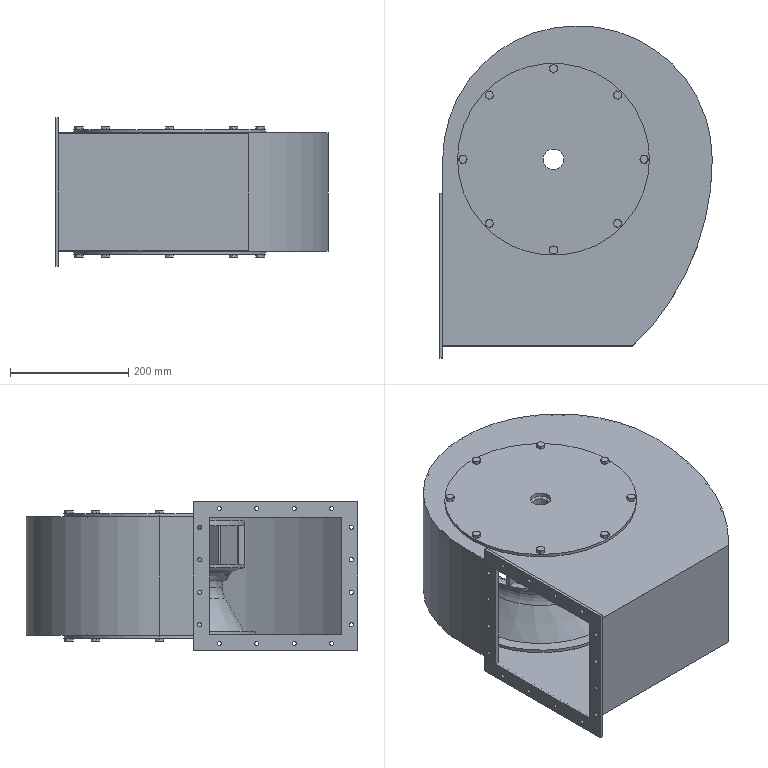Part | SolidWorks | features Boss 6, Revolution 3, CirPattern 2, Cut 2, Extrusion 1, ICE 1, MirrorPattern 1, RevCut 1, Shell 1 | 1 solid | 439 faces | box 460 x 560.054 x 251 mm | volume 3395369 mm3 | plane 233 | cone 102 | cylinder 90 | torus 14 | commonest cylinder face diameters 7 x32 74.4 x32 324 x6 35 x4 285.774 x4 45 x2